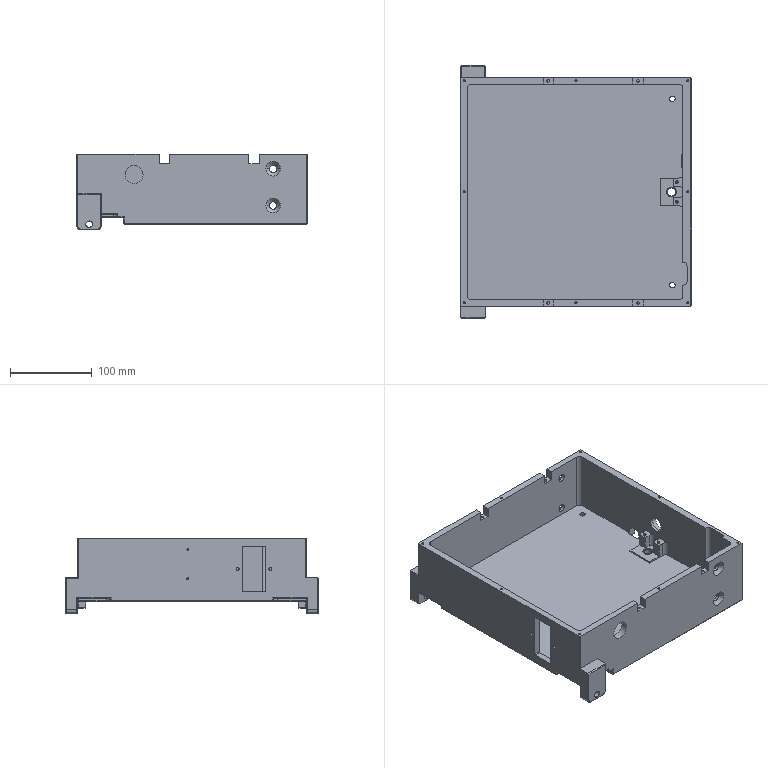NC program | Mastercam | posted with a generic post
Lines 47 to 692 of 104433:
(50 FEM |TOOL - 23|DIA. OFF. - 23|LEN. - 23|TOOL DIA. - 50.)
N158 T23 M6
N160 G0 G54 G90 X144. Y-196.5 C0. B0. S4000 M3
N162 G43 H23 Z50.
N164 Z1.
N166 G1 Z0. F600.
N168 Y-171.5 F4000.
N170 G3 X139. Y-166.5 I-5.
N172 G1 X-139. Z-.217
N174 G2 X-157.031 Y-159.031 Z-.232 J25.5
N176 G1 X-158.031 Y-158.031 Z-.234
N178 G2 X-165.5 Y-140. Z-.249 I18.031 J18.031
N180 G1 Y140. Z-.468
N182 G2 X-158.031 Y158.031 Z-.483 I25.5
N184 G1 X-157.031 Y159.031 Z-.484
N186 G2 X-139. Y166.5 Z-.5 I18.031 J-18.031
N188 G1 X139. Z-.717
N190 G2 X157.031 Y159.031 Z-.732 J-25.5
N192 G1 X158.031 Y158.031 Z-.734
N194 G2 X165.5 Y140. Z-.749 I-18.031 J-18.031
N196 G1 Y-140. Z-.968
N198 G2 X158.031 Y-158.031 Z-.983 I-25.5
N200 G1 X157.031 Y-159.031 Z-.984
N202 G2 X139. Y-166.5 Z-1. I-18.031 J18.031
N204 G1 X-139. Z-1.217
N206 G2 X-157.031 Y-159.031 Z-1.232 J25.5
N208 G1 X-158.031 Y-158.031 Z-1.234
N210 G2 X-165.5 Y-140. Z-1.249 I18.031 J18.031
N212 G1 Y140. Z-1.468
N214 G2 X-158.031 Y158.031 Z-1.483 I25.5
N216 G1 X-157.031 Y159.031 Z-1.484
N218 G2 X-139. Y166.5 Z-1.5 I18.031 J-18.031
N220 G1 X139. Z-1.717
N222 G2 X157.031 Y159.031 Z-1.732 J-25.5
N224 G1 X158.031 Y158.031 Z-1.734
N226 G2 X165.5 Y140. Z-1.749 I-18.031 J-18.031
N228 G1 Y-140. Z-1.968
N230 G2 X158.031 Y-158.031 Z-1.983 I-25.5
N232 G1 X157.031 Y-159.031 Z-1.984
N234 G2 X139. Y-166.5 Z-2. I-18.031 J18.031
N236 G1 X-139. Z-2.217
N238 G2 X-157.031 Y-159.031 Z-2.232 J25.5
N240 G1 X-158.031 Y-158.031 Z-2.234
N242 G2 X-165.5 Y-140. Z-2.249 I18.031 J18.031
N244 G1 Y140. Z-2.468
N246 G2 X-158.031 Y158.031 Z-2.483 I25.5
N248 G1 X-157.031 Y159.031 Z-2.484
N250 G2 X-139. Y166.5 Z-2.5 I18.031 J-18.031
N252 G1 X139. Z-2.717
N254 G2 X157.031 Y159.031 Z-2.732 J-25.5
N256 G1 X158.031 Y158.031 Z-2.734
N258 G2 X165.5 Y140. Z-2.749 I-18.031 J-18.031
N260 G1 Y-140. Z-2.968
N262 G2 X158.031 Y-158.031 Z-2.983 I-25.5
N264 G1 X157.031 Y-159.031 Z-2.984
N266 G2 X139. Y-166.5 Z-3. I-18.031 J18.031
N268 G1 X-139. Z-3.217
N270 G2 X-157.031 Y-159.031 Z-3.232 J25.5
N272 G1 X-158.031 Y-158.031 Z-3.234
N274 G2 X-165.5 Y-140. Z-3.249 I18.031 J18.031
N276 G1 Y140. Z-3.468
N278 G2 X-158.031 Y158.031 Z-3.483 I25.5
N280 G1 X-157.031 Y159.031 Z-3.484
N282 G2 X-139. Y166.5 Z-3.5 I18.031 J-18.031
N284 G1 X139. Z-3.717
N286 G2 X157.031 Y159.031 Z-3.732 J-25.5
N288 G1 X158.031 Y158.031 Z-3.734
N290 G2 X165.5 Y140. Z-3.749 I-18.031 J-18.031
N292 G1 Y-140. Z-3.968
N294 G2 X158.031 Y-158.031 Z-3.983 I-25.5
N296 G1 X157.031 Y-159.031 Z-3.984
N298 G2 X139. Y-166.5 Z-4. I-18.031 J18.031
N300 G1 X-139. Z-4.217
N302 G2 X-157.031 Y-159.031 Z-4.232 J25.5
N304 G1 X-158.031 Y-158.031 Z-4.234
N306 G2 X-165.5 Y-140. Z-4.249 I18.031 J18.031
N308 G1 Y140. Z-4.468
N310 G2 X-158.031 Y158.031 Z-4.483 I25.5
N312 G1 X-157.031 Y159.031 Z-4.484
N314 G2 X-139. Y166.5 Z-4.5 I18.031 J-18.031
N316 G1 X139. Z-4.717
N318 G2 X157.031 Y159.031 Z-4.732 J-25.5
N320 G1 X158.031 Y158.031 Z-4.734
N322 G2 X165.5 Y140. Z-4.749 I-18.031 J-18.031
N324 G1 Y-140. Z-4.968
N326 G2 X158.031 Y-158.031 Z-4.983 I-25.5
N328 G1 X157.031 Y-159.031 Z-4.984
N330 G2 X139. Y-166.5 Z-5. I-18.031 J18.031
N332 G1 X-139. Z-5.217
N334 G2 X-157.031 Y-159.031 Z-5.232 J25.5
N336 G1 X-158.031 Y-158.031 Z-5.234
N338 G2 X-165.5 Y-140. Z-5.249 I18.031 J18.031
N340 G1 Y140. Z-5.468
N342 G2 X-158.031 Y158.031 Z-5.483 I25.5
N344 G1 X-157.031 Y159.031 Z-5.484
N346 G2 X-139. Y166.5 Z-5.5 I18.031 J-18.031
N348 G1 X139. Z-5.717
N350 G2 X157.031 Y159.031 Z-5.732 J-25.5
N352 G1 X158.031 Y158.031 Z-5.734
N354 G2 X165.5 Y140. Z-5.749 I-18.031 J-18.031
N356 G1 Y-140. Z-5.968
N358 G2 X158.031 Y-158.031 Z-5.983 I-25.5
N360 G1 X157.031 Y-159.031 Z-5.984
N362 G2 X139. Y-166.5 Z-6. I-18.031 J18.031
N364 G1 X-139. Z-6.217
N366 G2 X-157.031 Y-159.031 Z-6.232 J25.5
N368 G1 X-158.031 Y-158.031 Z-6.234
N370 G2 X-165.5 Y-140. Z-6.249 I18.031 J18.031
N372 G1 Y140. Z-6.468
N374 G2 X-158.031 Y158.031 Z-6.483 I25.5
N376 G1 X-157.031 Y159.031 Z-6.484
N378 G2 X-139. Y166.5 Z-6.5 I18.031 J-18.031
N380 G1 X139. Z-6.717
N382 G2 X157.031 Y159.031 Z-6.732 J-25.5
N384 G1 X158.031 Y158.031 Z-6.734
N386 G2 X165.5 Y140. Z-6.749 I-18.031 J-18.031
N388 G1 Y-140. Z-6.968
N390 G2 X158.031 Y-158.031 Z-6.983 I-25.5
N392 G1 X157.031 Y-159.031 Z-6.984
N394 G2 X139. Y-166.5 Z-7. I-18.031 J18.031
N396 G1 X-139. Z-7.217
N398 G2 X-157.031 Y-159.031 Z-7.232 J25.5
N400 G1 X-158.031 Y-158.031 Z-7.234
N402 G2 X-165.5 Y-140. Z-7.249 I18.031 J18.031
N404 G1 Y140. Z-7.468
N406 G2 X-158.031 Y158.031 Z-7.483 I25.5
N408 G1 X-157.031 Y159.031 Z-7.484
N410 G2 X-139. Y166.5 Z-7.5 I18.031 J-18.031
N412 G1 X139. Z-7.717
N414 G2 X157.031 Y159.031 Z-7.732 J-25.5
N416 G1 X158.031 Y158.031 Z-7.734
N418 G2 X165.5 Y140. Z-7.749 I-18.031 J-18.031
N420 G1 Y-140. Z-7.968
N422 G2 X158.031 Y-158.031 Z-7.983 I-25.5
N424 G1 X157.031 Y-159.031 Z-7.984
N426 G2 X139. Y-166.5 Z-8. I-18.031 J18.031
N428 G1 X-139. Z-8.217
N430 G2 X-157.031 Y-159.031 Z-8.232 J25.5
N432 G1 X-158.031 Y-158.031 Z-8.234
N434 G2 X-165.5 Y-140. Z-8.249 I18.031 J18.031
N436 G1 Y140. Z-8.468
N438 G2 X-158.031 Y158.031 Z-8.483 I25.5
N440 G1 X-157.031 Y159.031 Z-8.484
N442 G2 X-139. Y166.5 Z-8.5 I18.031 J-18.031
N444 G1 X139. Z-8.717
N446 G2 X157.031 Y159.031 Z-8.732 J-25.5
N448 G1 X158.031 Y158.031 Z-8.734
N450 G2 X165.5 Y140. Z-8.749 I-18.031 J-18.031
N452 G1 Y-140. Z-8.968
N454 G2 X158.031 Y-158.031 Z-8.983 I-25.5
N456 G1 X157.031 Y-159.031 Z-8.984
N458 G2 X139. Y-166.5 Z-9. I-18.031 J18.031
N460 G1 X-139. Z-9.217
N462 G2 X-157.031 Y-159.031 Z-9.232 J25.5
N464 G1 X-158.031 Y-158.031 Z-9.234
N466 G2 X-165.5 Y-140. Z-9.249 I18.031 J18.031
N468 G1 Y140. Z-9.468
N470 G2 X-158.031 Y158.031 Z-9.483 I25.5
N472 G1 X-157.031 Y159.031 Z-9.484
N474 G2 X-139. Y166.5 Z-9.5 I18.031 J-18.031
N476 G1 X139. Z-9.717
N478 G2 X157.031 Y159.031 Z-9.732 J-25.5
N480 G1 X158.031 Y158.031 Z-9.734
N482 G2 X165.5 Y140. Z-9.749 I-18.031 J-18.031
N484 G1 Y-140. Z-9.968
N486 G2 X158.031 Y-158.031 Z-9.983 I-25.5
N488 G1 X157.031 Y-159.031 Z-9.984
N490 G2 X139. Y-166.5 Z-10. I-18.031 J18.031
N492 G1 X-139. Z-10.217
N494 G2 X-157.031 Y-159.031 Z-10.232 J25.5
N496 G1 X-158.031 Y-158.031 Z-10.234
N498 G2 X-165.5 Y-140. Z-10.249 I18.031 J18.031
N500 G1 Y140. Z-10.468
N502 G2 X-158.031 Y158.031 Z-10.483 I25.5
N504 G1 X-157.031 Y159.031 Z-10.484
N506 G2 X-139. Y166.5 Z-10.5 I18.031 J-18.031
N508 G1 X139. Z-10.717
N510 G2 X157.031 Y159.031 Z-10.732 J-25.5
N512 G1 X158.031 Y158.031 Z-10.734
N514 G2 X165.5 Y140. Z-10.749 I-18.031 J-18.031
N516 G1 Y-140. Z-10.968
N518 G2 X158.031 Y-158.031 Z-10.983 I-25.5
N520 G1 X157.031 Y-159.031 Z-10.984
N522 G2 X139. Y-166.5 Z-11. I-18.031 J18.031
N524 G1 X-139. Z-11.217
N526 G2 X-157.031 Y-159.031 Z-11.232 J25.5
N528 G1 X-158.031 Y-158.031 Z-11.234
N530 G2 X-165.5 Y-140. Z-11.249 I18.031 J18.031
N532 G1 Y140. Z-11.468
N534 G2 X-158.031 Y158.031 Z-11.483 I25.5
N536 G1 X-157.031 Y159.031 Z-11.484
N538 G2 X-139. Y166.5 Z-11.5 I18.031 J-18.031
N540 G1 X139. Z-11.717
N542 G2 X157.031 Y159.031 Z-11.732 J-25.5
N544 G1 X158.031 Y158.031 Z-11.734
N546 G2 X165.5 Y140. Z-11.749 I-18.031 J-18.031
N548 G1 Y-140. Z-11.968
N550 G2 X158.031 Y-158.031 Z-11.983 I-25.5
N552 G1 X157.031 Y-159.031 Z-11.984
N554 G2 X139. Y-166.5 Z-12. I-18.031 J18.031
N556 G1 X-139. Z-12.217
N558 G2 X-157.031 Y-159.031 Z-12.232 J25.5
N560 G1 X-158.031 Y-158.031 Z-12.234
N562 G2 X-165.5 Y-140. Z-12.249 I18.031 J18.031
N564 G1 Y140. Z-12.468
N566 G2 X-158.031 Y158.031 Z-12.483 I25.5
N568 G1 X-157.031 Y159.031 Z-12.484
N570 G2 X-139. Y166.5 Z-12.5 I18.031 J-18.031
N572 G1 X139. Z-12.717
N574 G2 X157.031 Y159.031 Z-12.732 J-25.5
N576 G1 X158.031 Y158.031 Z-12.734
N578 G2 X165.5 Y140. Z-12.749 I-18.031 J-18.031
N580 G1 Y-140. Z-12.968
N582 G2 X158.031 Y-158.031 Z-12.983 I-25.5
N584 G1 X157.031 Y-159.031 Z-12.984
N586 G2 X139. Y-166.5 Z-13. I-18.031 J18.031
N588 G1 X-139. Z-13.217
N590 G2 X-157.031 Y-159.031 Z-13.232 J25.5
N592 G1 X-158.031 Y-158.031 Z-13.234
N594 G2 X-165.5 Y-140. Z-13.249 I18.031 J18.031
N596 G1 Y140. Z-13.468
N598 G2 X-158.031 Y158.031 Z-13.483 I25.5
N600 G1 X-157.031 Y159.031 Z-13.484
N602 G2 X-139. Y166.5 Z-13.5 I18.031 J-18.031
N604 G1 X139. Z-13.717
N606 G2 X157.031 Y159.031 Z-13.732 J-25.5
N608 G1 X158.031 Y158.031 Z-13.734
N610 G2 X165.5 Y140. Z-13.749 I-18.031 J-18.031
N612 G1 Y-140. Z-13.968
N614 G2 X158.031 Y-158.031 Z-13.983 I-25.5
N616 G1 X157.031 Y-159.031 Z-13.984
N618 G2 X139. Y-166.5 Z-14. I-18.031 J18.031
N620 G1 X-139. Z-14.217
N622 G2 X-157.031 Y-159.031 Z-14.232 J25.5
N624 G1 X-158.031 Y-158.031 Z-14.234
N626 G2 X-165.5 Y-140. Z-14.249 I18.031 J18.031
N628 G1 Y140. Z-14.468
N630 G2 X-158.031 Y158.031 Z-14.483 I25.5
N632 G1 X-157.031 Y159.031 Z-14.484
N634 G2 X-139. Y166.5 Z-14.5 I18.031 J-18.031
N636 G1 X139. Z-14.717
N638 G2 X157.031 Y159.031 Z-14.732 J-25.5
N640 G1 X158.031 Y158.031 Z-14.734
N642 G2 X165.5 Y140. Z-14.749 I-18.031 J-18.031
N644 G1 Y-140. Z-14.968
N646 G2 X158.031 Y-158.031 Z-14.983 I-25.5
N648 G1 X157.031 Y-159.031 Z-14.984
N650 G2 X139. Y-166.5 Z-15. I-18.031 J18.031
N652 G1 X-139. Z-15.217
N654 G2 X-157.031 Y-159.031 Z-15.232 J25.5
N656 G1 X-158.031 Y-158.031 Z-15.234
N658 G2 X-165.5 Y-140. Z-15.249 I18.031 J18.031
N660 G1 Y140. Z-15.468
N662 G2 X-158.031 Y158.031 Z-15.483 I25.5
N664 G1 X-157.031 Y159.031 Z-15.484
N666 G2 X-139. Y166.5 Z-15.5 I18.031 J-18.031
N668 G1 X139. Z-15.717
N670 G2 X157.031 Y159.031 Z-15.732 J-25.5
N672 G1 X158.031 Y158.031 Z-15.734
N674 G2 X165.5 Y140. Z-15.749 I-18.031 J-18.031
N676 G1 Y-140. Z-15.968
N678 G2 X158.031 Y-158.031 Z-15.983 I-25.5
N680 G1 X157.031 Y-159.031 Z-15.984
N682 G2 X139. Y-166.5 Z-16. I-18.031 J18.031
N684 G1 X-139. Z-16.217
N686 G2 X-157.031 Y-159.031 Z-16.232 J25.5
N688 G1 X-158.031 Y-158.031 Z-16.234
N690 G2 X-165.5 Y-140. Z-16.249 I18.031 J18.031
N692 G1 Y140. Z-16.468
N694 G2 X-158.031 Y158.031 Z-16.483 I25.5
N696 G1 X-157.031 Y159.031 Z-16.484
N698 G2 X-139. Y166.5 Z-16.5 I18.031 J-18.031
N700 G1 X139. Z-16.717
N702 G2 X157.031 Y159.031 Z-16.732 J-25.5
N704 G1 X158.031 Y158.031 Z-16.734
N706 G2 X165.5 Y140. Z-16.749 I-18.031 J-18.031
N708 G1 Y-140. Z-16.968
N710 G2 X158.031 Y-158.031 Z-16.983 I-25.5
N712 G1 X157.031 Y-159.031 Z-16.984
N714 G2 X139. Y-166.5 Z-17. I-18.031 J18.031
N716 G1 X-139. Z-17.217
N718 G2 X-157.031 Y-159.031 Z-17.232 J25.5
N720 G1 X-158.031 Y-158.031 Z-17.234
N722 G2 X-165.5 Y-140. Z-17.249 I18.031 J18.031
N724 G1 Y140. Z-17.468
N726 G2 X-158.031 Y158.031 Z-17.483 I25.5
N728 G1 X-157.031 Y159.031 Z-17.484
N730 G2 X-139. Y166.5 Z-17.5 I18.031 J-18.031
N732 G1 X139. Z-17.717
N734 G2 X157.031 Y159.031 Z-17.732 J-25.5
N736 G1 X158.031 Y158.031 Z-17.734
N738 G2 X165.5 Y140. Z-17.749 I-18.031 J-18.031
N740 G1 Y-140. Z-17.968
N742 G2 X158.031 Y-158.031 Z-17.983 I-25.5
N744 G1 X157.031 Y-159.031 Z-17.984
N746 G2 X139. Y-166.5 Z-18. I-18.031 J18.031
N748 G1 X-139. Z-18.217
N750 G2 X-157.031 Y-159.031 Z-18.232 J25.5
N752 G1 X-158.031 Y-158.031 Z-18.234
N754 G2 X-165.5 Y-140. Z-18.249 I18.031 J18.031
N756 G1 Y140. Z-18.468
N758 G2 X-158.031 Y158.031 Z-18.483 I25.5
N760 G1 X-157.031 Y159.031 Z-18.484
N762 G2 X-139. Y166.5 Z-18.5 I18.031 J-18.031
N764 G1 X139. Z-18.717
N766 G2 X157.031 Y159.031 Z-18.732 J-25.5
N768 G1 X158.031 Y158.031 Z-18.734
N770 G2 X165.5 Y140. Z-18.749 I-18.031 J-18.031
N772 G1 Y-140. Z-18.968
N774 G2 X158.031 Y-158.031 Z-18.983 I-25.5
N776 G1 X157.031 Y-159.031 Z-18.984
N778 G2 X139. Y-166.5 Z-19. I-18.031 J18.031
N780 G1 X-139. Z-19.217
N782 G2 X-157.031 Y-159.031 Z-19.232 J25.5
N784 G1 X-158.031 Y-158.031 Z-19.234
N786 G2 X-165.5 Y-140. Z-19.249 I18.031 J18.031
N788 G1 Y140. Z-19.468
N790 G2 X-158.031 Y158.031 Z-19.483 I25.5
N792 G1 X-157.031 Y159.031 Z-19.484
N794 G2 X-139. Y166.5 Z-19.5 I18.031 J-18.031
N796 G1 X139. Z-19.717
N798 G2 X157.031 Y159.031 Z-19.732 J-25.5
N800 G1 X158.031 Y158.031 Z-19.734
N802 G2 X165.5 Y140. Z-19.749 I-18.031 J-18.031
N804 G1 Y-140. Z-19.968
N806 G2 X158.031 Y-158.031 Z-19.983 I-25.5
N808 G1 X157.031 Y-159.031 Z-19.984
N810 G2 X139. Y-166.5 Z-20. I-18.031 J18.031
N812 G1 X-139. Z-20.217
N814 G2 X-157.031 Y-159.031 Z-20.232 J25.5
N816 G1 X-158.031 Y-158.031 Z-20.234
N818 G2 X-165.5 Y-140. Z-20.249 I18.031 J18.031
N820 G1 Y140. Z-20.468
N822 G2 X-158.031 Y158.031 Z-20.483 I25.5
N824 G1 X-157.031 Y159.031 Z-20.484
N826 G2 X-139. Y166.5 Z-20.5 I18.031 J-18.031
N828 G1 X139. Z-20.717
N830 G2 X157.031 Y159.031 Z-20.732 J-25.5
N832 G1 X158.031 Y158.031 Z-20.734
N834 G2 X165.5 Y140. Z-20.749 I-18.031 J-18.031
N836 G1 Y-140. Z-20.968
N838 G2 X158.031 Y-158.031 Z-20.983 I-25.5
N840 G1 X157.031 Y-159.031 Z-20.984
N842 G2 X139. Y-166.5 Z-21. I-18.031 J18.031
N844 G1 X-139. Z-21.217
N846 G2 X-157.031 Y-159.031 Z-21.232 J25.5
N848 G1 X-158.031 Y-158.031 Z-21.234
N850 G2 X-165.5 Y-140. Z-21.249 I18.031 J18.031
N852 G1 Y140. Z-21.468
N854 G2 X-158.031 Y158.031 Z-21.483 I25.5
N856 G1 X-157.031 Y159.031 Z-21.484
N858 G2 X-139. Y166.5 Z-21.5 I18.031 J-18.031
N860 G1 X139. Z-21.717
N862 G2 X157.031 Y159.031 Z-21.732 J-25.5
N864 G1 X158.031 Y158.031 Z-21.734
N866 G2 X165.5 Y140. Z-21.749 I-18.031 J-18.031
N868 G1 Y-140. Z-21.968
N870 G2 X158.031 Y-158.031 Z-21.983 I-25.5
N872 G1 X157.031 Y-159.031 Z-21.984
N874 G2 X139. Y-166.5 Z-22. I-18.031 J18.031
N876 G1 X-139. Z-22.217
N878 G2 X-157.031 Y-159.031 Z-22.232 J25.5
N880 G1 X-158.031 Y-158.031 Z-22.234
N882 G2 X-165.5 Y-140. Z-22.249 I18.031 J18.031
N884 G1 Y140. Z-22.468
N886 G2 X-158.031 Y158.031 Z-22.483 I25.5
N888 G1 X-157.031 Y159.031 Z-22.484
N890 G2 X-139. Y166.5 Z-22.5 I18.031 J-18.031
N892 G1 X139. Z-22.717
N894 G2 X157.031 Y159.031 Z-22.732 J-25.5
N896 G1 X158.031 Y158.031 Z-22.734
N898 G2 X165.5 Y140. Z-22.749 I-18.031 J-18.031
N900 G1 Y-140. Z-22.968
N902 G2 X158.031 Y-158.031 Z-22.983 I-25.5
N904 G1 X157.031 Y-159.031 Z-22.984
N906 G2 X139. Y-166.5 Z-23. I-18.031 J18.031
N908 G1 X-139. Z-23.217
N910 G2 X-157.031 Y-159.031 Z-23.232 J25.5
N912 G1 X-158.031 Y-158.031 Z-23.234
N914 G2 X-165.5 Y-140. Z-23.249 I18.031 J18.031
N916 G1 Y140. Z-23.468
N918 G2 X-158.031 Y158.031 Z-23.483 I25.5
N920 G1 X-157.031 Y159.031 Z-23.484
N922 G2 X-139. Y166.5 Z-23.5 I18.031 J-18.031
N924 G1 X139. Z-23.717
N926 G2 X157.031 Y159.031 Z-23.732 J-25.5
N928 G1 X158.031 Y158.031 Z-23.734
N930 G2 X165.5 Y140. Z-23.749 I-18.031 J-18.031
N932 G1 Y-140. Z-23.968
N934 G2 X158.031 Y-158.031 Z-23.983 I-25.5
N936 G1 X157.031 Y-159.031 Z-23.984
N938 G2 X139. Y-166.5 Z-24. I-18.031 J18.031
N940 G1 X-139. Z-24.217
N942 G2 X-157.031 Y-159.031 Z-24.232 J25.5
N944 G1 X-158.031 Y-158.031 Z-24.234
N946 G2 X-165.5 Y-140. Z-24.249 I18.031 J18.031
N948 G1 Y140. Z-24.468
N950 G2 X-158.031 Y158.031 Z-24.483 I25.5
N952 G1 X-157.031 Y159.031 Z-24.484
N954 G2 X-139. Y166.5 Z-24.5 I18.031 J-18.031
N956 G1 X139. Z-24.717
N958 G2 X157.031 Y159.031 Z-24.732 J-25.5
N960 G1 X158.031 Y158.031 Z-24.734
N962 G2 X165.5 Y140. Z-24.749 I-18.031 J-18.031
N964 G1 Y-140. Z-24.968
N966 G2 X158.031 Y-158.031 Z-24.983 I-25.5
N968 G1 X157.031 Y-159.031 Z-24.984
N970 G2 X139. Y-166.5 Z-25. I-18.031 J18.031
N972 G1 X-139. Z-25.217
N974 G2 X-157.031 Y-159.031 Z-25.232 J25.5
N976 G1 X-158.031 Y-158.031 Z-25.234
N978 G2 X-165.5 Y-140. Z-25.249 I18.031 J18.031
N980 G1 Y140. Z-25.468
N982 G2 X-158.031 Y158.031 Z-25.483 I25.5
N984 G1 X-157.031 Y159.031 Z-25.484
N986 G2 X-139. Y166.5 Z-25.5 I18.031 J-18.031
N988 G1 X139. Z-25.717
N990 G2 X157.031 Y159.031 Z-25.732 J-25.5
N992 G1 X158.031 Y158.031 Z-25.734
N994 G2 X165.5 Y140. Z-25.749 I-18.031 J-18.031
N996 G1 Y-140. Z-25.968
N998 G2 X158.031 Y-158.031 Z-25.983 I-25.5
N1000 G1 X157.031 Y-159.031 Z-25.984
N1002 G2 X139. Y-166.5 Z-26. I-18.031 J18.031
N1004 G1 X-139. Z-26.217
N1006 G2 X-157.031 Y-159.031 Z-26.232 J25.5
N1008 G1 X-158.031 Y-158.031 Z-26.234
N1010 G2 X-165.5 Y-140. Z-26.249 I18.031 J18.031
N1012 G1 Y140. Z-26.468
N1014 G2 X-158.031 Y158.031 Z-26.483 I25.5
N1016 G1 X-157.031 Y159.031 Z-26.484
N1018 G2 X-139. Y166.5 Z-26.5 I18.031 J-18.031
N1020 G1 X139. Z-26.717
N1022 G2 X157.031 Y159.031 Z-26.732 J-25.5
N1024 G1 X158.031 Y158.031 Z-26.734
N1026 G2 X165.5 Y140. Z-26.749 I-18.031 J-18.031
N1028 G1 Y-140. Z-26.968
N1030 G2 X158.031 Y-158.031 Z-26.983 I-25.5
N1032 G1 X157.031 Y-159.031 Z-26.984
N1034 G2 X139. Y-166.5 Z-27. I-18.031 J18.031
N1036 G1 X-139. Z-27.217
N1038 G2 X-157.031 Y-159.031 Z-27.232 J25.5
N1040 G1 X-158.031 Y-158.031 Z-27.234
N1042 G2 X-165.5 Y-140. Z-27.249 I18.031 J18.031
N1044 G1 Y140. Z-27.468
N1046 G2 X-158.031 Y158.031 Z-27.483 I25.5
N1048 G1 X-157.031 Y159.031 Z-27.484
N1050 G2 X-139. Y166.5 Z-27.5 I18.031 J-18.031
N1052 G1 X139. Z-27.717
N1054 G2 X157.031 Y159.031 Z-27.732 J-25.5
N1056 G1 X158.031 Y158.031 Z-27.734
N1058 G2 X165.5 Y140. Z-27.749 I-18.031 J-18.031
N1060 G1 Y-140. Z-27.968
N1062 G2 X158.031 Y-158.031 Z-27.983 I-25.5
N1064 G1 X157.031 Y-159.031 Z-27.984
N1066 G2 X139. Y-166.5 Z-28. I-18.031 J18.031
N1068 G1 X-139. Z-28.217
N1070 G2 X-157.031 Y-159.031 Z-28.232 J25.5
N1072 G1 X-158.031 Y-158.031 Z-28.234
N1074 G2 X-165.5 Y-140. Z-28.249 I18.031 J18.031
N1076 G1 Y140. Z-28.468
N1078 G2 X-158.031 Y158.031 Z-28.483 I25.5
N1080 G1 X-157.031 Y159.031 Z-28.484
N1082 G2 X-139. Y166.5 Z-28.5 I18.031 J-18.031
N1084 G1 X139. Z-28.717
N1086 G2 X157.031 Y159.031 Z-28.732 J-25.5
N1088 G1 X158.031 Y158.031 Z-28.734
N1090 G2 X165.5 Y140. Z-28.749 I-18.031 J-18.031
N1092 G1 Y-140. Z-28.968
N1094 G2 X158.031 Y-158.031 Z-28.983 I-25.5
N1096 G1 X157.031 Y-159.031 Z-28.984
N1098 G2 X139. Y-166.5 Z-29. I-18.031 J18.031
N1100 G1 X-139. Z-29.217
N1102 G2 X-157.031 Y-159.031 Z-29.232 J25.5
N1104 G1 X-158.031 Y-158.031 Z-29.234
N1106 G2 X-165.5 Y-140. Z-29.249 I18.031 J18.031
N1108 G1 Y140. Z-29.468
N1110 G2 X-158.031 Y158.031 Z-29.483 I25.5
N1112 G1 X-157.031 Y159.031 Z-29.484
N1114 G2 X-139. Y166.5 Z-29.5 I18.031 J-18.031
N1116 G1 X139. Z-29.717
N1118 G2 X157.031 Y159.031 Z-29.732 J-25.5
N1120 G1 X158.031 Y158.031 Z-29.734
N1122 G2 X165.5 Y140. Z-29.749 I-18.031 J-18.031
N1124 G1 Y-140. Z-29.968
N1126 G2 X158.031 Y-158.031 Z-29.983 I-25.5
N1128 G1 X157.031 Y-159.031 Z-29.984
N1130 G2 X139. Y-166.5 Z-30. I-18.031 J18.031
N1132 G1 X-139. Z-30.217
N1134 G2 X-157.031 Y-159.031 Z-30.232 J25.5
N1136 G1 X-158.031 Y-158.031 Z-30.234
N1138 G2 X-165.5 Y-140. Z-30.249 I18.031 J18.031
N1140 G1 Y140. Z-30.468
N1142 G2 X-158.031 Y158.031 Z-30.483 I25.5
N1144 G1 X-157.031 Y159.031 Z-30.484
N1146 G2 X-139. Y166.5 Z-30.5 I18.031 J-18.031
N1148 G1 X139. Z-30.717
N1150 G2 X157.031 Y159.031 Z-30.732 J-25.5
N1152 G1 X158.031 Y158.031 Z-30.734
N1154 G2 X165.5 Y140. Z-30.749 I-18.031 J-18.031
N1156 G1 Y-140. Z-30.968
N1158 G2 X158.031 Y-158.031 Z-30.983 I-25.5
N1160 G1 X157.031 Y-159.031 Z-30.984
N1162 G2 X139. Y-166.5 Z-31. I-18.031 J18.031
N1164 G1 X-139. Z-31.217
N1166 G2 X-157.031 Y-159.031 Z-31.232 J25.5
N1168 G1 X-158.031 Y-158.031 Z-31.234
N1170 G2 X-165.5 Y-140. Z-31.249 I18.031 J18.031
N1172 G1 Y140. Z-31.468
N1174 G2 X-158.031 Y158.031 Z-31.483 I25.5
N1176 G1 X-157.031 Y159.031 Z-31.484
N1178 G2 X-139. Y166.5 Z-31.5 I18.031 J-18.031
N1180 G1 X139. Z-31.717
N1182 G2 X157.031 Y159.031 Z-31.732 J-25.5
N1184 G1 X158.031 Y158.031 Z-31.734
N1186 G2 X165.5 Y140. Z-31.749 I-18.031 J-18.031
N1188 G1 Y-140. Z-31.968
N1190 G2 X158.031 Y-158.031 Z-31.983 I-25.5
N1192 G1 X157.031 Y-159.031 Z-31.984
N1194 G2 X139. Y-166.5 Z-32. I-18.031 J18.031
N1196 G1 X-139. Z-32.217
N1198 G2 X-157.031 Y-159.031 Z-32.232 J25.5
N1200 G1 X-158.031 Y-158.031 Z-32.234
N1202 G2 X-165.5 Y-140. Z-32.249 I18.031 J18.031
N1204 G1 Y140. Z-32.468
N1206 G2 X-158.031 Y158.031 Z-32.483 I25.5
N1208 G1 X-157.031 Y159.031 Z-32.484
N1210 G2 X-139. Y166.5 Z-32.5 I18.031 J-18.031
N1212 G1 X139. Z-32.717
N1214 G2 X157.031 Y159.031 Z-32.732 J-25.5
N1216 G1 X158.031 Y158.031 Z-32.734
N1218 G2 X165.5 Y140. Z-32.749 I-18.031 J-18.031
N1220 G1 Y-140. Z-32.968
N1222 G2 X158.031 Y-158.031 Z-32.983 I-25.5
N1224 G1 X157.031 Y-159.031 Z-32.984
N1226 G2 X139. Y-166.5 Z-33. I-18.031 J18.031
N1228 G1 X-139. Z-33.217
N1230 G2 X-157.031 Y-159.031 Z-33.232 J25.5
N1232 G1 X-158.031 Y-158.031 Z-33.234
N1234 G2 X-165.5 Y-140. Z-33.249 I18.031 J18.031
N1236 G1 Y140. Z-33.468
N1238 G2 X-158.031 Y158.031 Z-33.483 I25.5
N1240 G1 X-157.031 Y159.031 Z-33.484
N1242 G2 X-139. Y166.5 Z-33.5 I18.031 J-18.031
N1244 G1 X139. Z-33.717
N1246 G2 X157.031 Y159.031 Z-33.732 J-25.5
N1248 G1 X158.031 Y158.031 Z-33.734
N1250 G2 X165.5 Y140. Z-33.749 I-18.031 J-18.031
N1252 G1 Y-140. Z-33.968
N1254 G2 X158.031 Y-158.031 Z-33.983 I-25.5
N1256 G1 X157.031 Y-159.031 Z-33.984
N1258 G2 X139. Y-166.5 Z-34. I-18.031 J18.031
N1260 G1 X-139. Z-34.217
N1262 G2 X-157.031 Y-159.031 Z-34.232 J25.5
N1264 G1 X-158.031 Y-158.031 Z-34.234
N1266 G2 X-165.5 Y-140. Z-34.249 I18.031 J18.031
N1268 G1 Y140. Z-34.468
N1270 G2 X-158.031 Y158.031 Z-34.483 I25.5
N1272 G1 X-157.031 Y159.031 Z-34.484
N1274 G2 X-139. Y166.5 Z-34.5 I18.031 J-18.031
N1276 G1 X139. Z-34.717
N1278 G2 X157.031 Y159.031 Z-34.732 J-25.5
N1280 G1 X158.031 Y158.031 Z-34.734
N1282 G2 X165.5 Y140. Z-34.749 I-18.031 J-18.031
N1284 G1 Y-140. Z-34.968
N1286 G2 X158.031 Y-158.031 Z-34.983 I-25.5
N1288 G1 X157.031 Y-159.031 Z-34.984
N1290 G2 X139. Y-166.5 Z-35. I-18.031 J18.031
N1292 G1 X-139. Z-35.217
N1294 G2 X-157.031 Y-159.031 Z-35.232 J25.5
N1296 G1 X-158.031 Y-158.031 Z-35.234
N1298 G2 X-165.5 Y-140. Z-35.249 I18.031 J18.031
N1300 G1 Y140. Z-35.468
N1302 G2 X-158.031 Y158.031 Z-35.483 I25.5
N1304 G1 X-157.031 Y159.031 Z-35.484
N1306 G2 X-139. Y166.5 Z-35.5 I18.031 J-18.031
N1308 G1 X139. Z-35.717
N1310 G2 X157.031 Y159.031 Z-35.732 J-25.5
N1312 G1 X158.031 Y158.031 Z-35.734
N1314 G2 X165.5 Y140. Z-35.749 I-18.031 J-18.031
N1316 G1 Y-140. Z-35.968
N1318 G2 X158.031 Y-158.031 Z-35.983 I-25.5
N1320 G1 X157.031 Y-159.031 Z-35.984
N1322 G2 X139. Y-166.5 Z-36. I-18.031 J18.031
N1324 G1 X-139. Z-36.217
N1326 G2 X-157.031 Y-159.031 Z-36.232 J25.5
N1328 G1 X-158.031 Y-158.031 Z-36.234
N1330 G2 X-165.5 Y-140. Z-36.249 I18.031 J18.031
N1332 G1 Y140. Z-36.468
N1334 G2 X-158.031 Y158.031 Z-36.483 I25.5
N1336 G1 X-157.031 Y159.031 Z-36.484
N1338 G2 X-139. Y166.5 Z-36.5 I18.031 J-18.031
N1340 G1 X139. Z-36.717
N1342 G2 X157.031 Y159.031 Z-36.732 J-25.5
N1344 G1 X158.031 Y158.031 Z-36.734
N1346 G2 X165.5 Y140. Z-36.749 I-18.031 J-18.031
N1348 G1 Y-140. Z-36.968
N1350 G2 X158.031 Y-158.031 Z-36.983 I-25.5
N1352 G1 X157.031 Y-159.031 Z-36.984
N1354 G2 X139. Y-166.5 Z-37. I-18.031 J18.031
N1356 G1 X-139. Z-37.217
N1358 G2 X-157.031 Y-159.031 Z-37.232 J25.5
N1360 G1 X-158.031 Y-158.031 Z-37.234
N1362 G2 X-165.5 Y-140. Z-37.249 I18.031 J18.031
N1364 G1 Y140. Z-37.468
N1366 G2 X-158.031 Y158.031 Z-37.483 I25.5
N1368 G1 X-157.031 Y159.031 Z-37.484
N1370 G2 X-139. Y166.5 Z-37.5 I18.031 J-18.031
N1372 G1 X139. Z-37.717
N1374 G2 X157.031 Y159.031 Z-37.732 J-25.5
N1376 G1 X158.031 Y158.031 Z-37.734
N1378 G2 X165.5 Y140. Z-37.749 I-18.031 J-18.031
N1380 G1 Y-140. Z-37.968
N1382 G2 X158.031 Y-158.031 Z-37.983 I-25.5
N1384 G1 X157.031 Y-159.031 Z-37.984
N1386 G2 X139. Y-166.5 Z-38. I-18.031 J18.031
N1388 G1 X-139. Z-38.217
N1390 G2 X-157.031 Y-159.031 Z-38.232 J25.5
N1392 G1 X-158.031 Y-158.031 Z-38.234
N1394 G2 X-165.5 Y-140. Z-38.249 I18.031 J18.031
N1396 G1 Y140. Z-38.468
N1398 G2 X-158.031 Y158.031 Z-38.483 I25.5
N1400 G1 X-157.031 Y159.031 Z-38.484
N1402 G2 X-139. Y166.5 Z-38.5 I18.031 J-18.031
N1404 G1 X139. Z-38.717
N1406 G2 X157.031 Y159.031 Z-38.732 J-25.5
N1408 G1 X158.031 Y158.031 Z-38.734
N1410 G2 X165.5 Y140. Z-38.749 I-18.031 J-18.031
N1412 G1 Y-140. Z-38.968
N1414 G2 X158.031 Y-158.031 Z-38.983 I-25.5
N1416 G1 X157.031 Y-159.031 Z-38.984
N1418 G2 X139. Y-166.5 Z-39. I-18.031 J18.031
N1420 G1 X-139. Z-39.217
N1422 G2 X-157.031 Y-159.031 Z-39.232 J25.5
N1424 G1 X-158.031 Y-158.031 Z-39.234
N1426 G2 X-165.5 Y-140. Z-39.249 I18.031 J18.031
N1428 G1 Y140. Z-39.468
N1430 G2 X-158.031 Y158.031 Z-39.483 I25.5
N1432 G1 X-157.031 Y159.031 Z-39.484
N1434 G2 X-139. Y166.5 Z-39.5 I18.031 J-18.031
N1436 G1 X139. Z-39.717
N1438 G2 X157.031 Y159.031 Z-39.732 J-25.5
N1440 G1 X158.031 Y158.031 Z-39.734
N1442 G2 X165.5 Y140. Z-39.749 I-18.031 J-18.031
N1444 G1 Y-140. Z-39.968
N1446 G2 X158.031 Y-158.031 Z-39.983 I-25.5